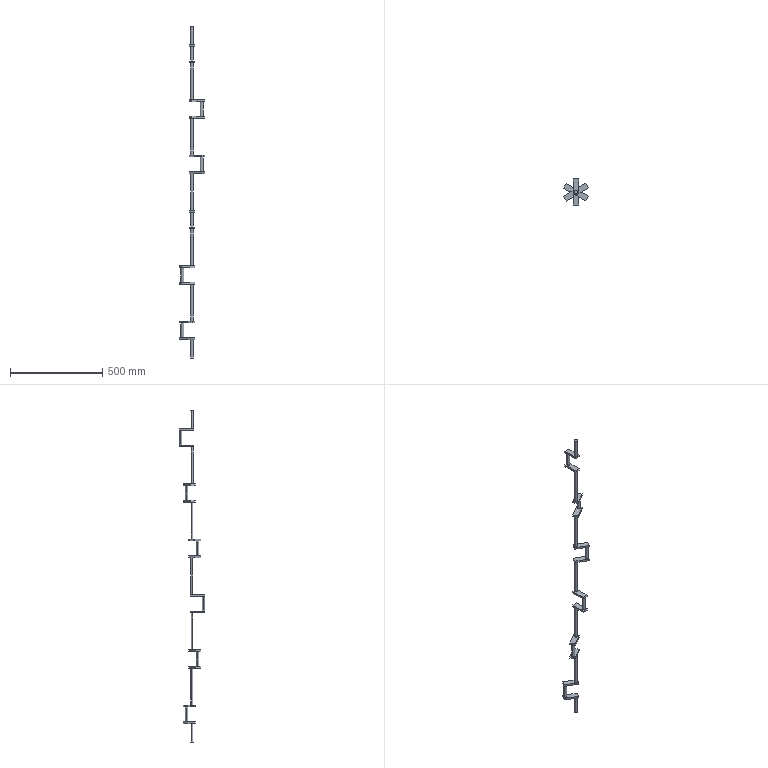Part | SolidWorks | features ICE 24, Extrusion 1 | 1 solid | 100 faces | box 136.244 x 140 x 1800 mm | volume 625784 mm3 | plane 74 | cylinder 26 | commonest cylinder face diameters 16 x26